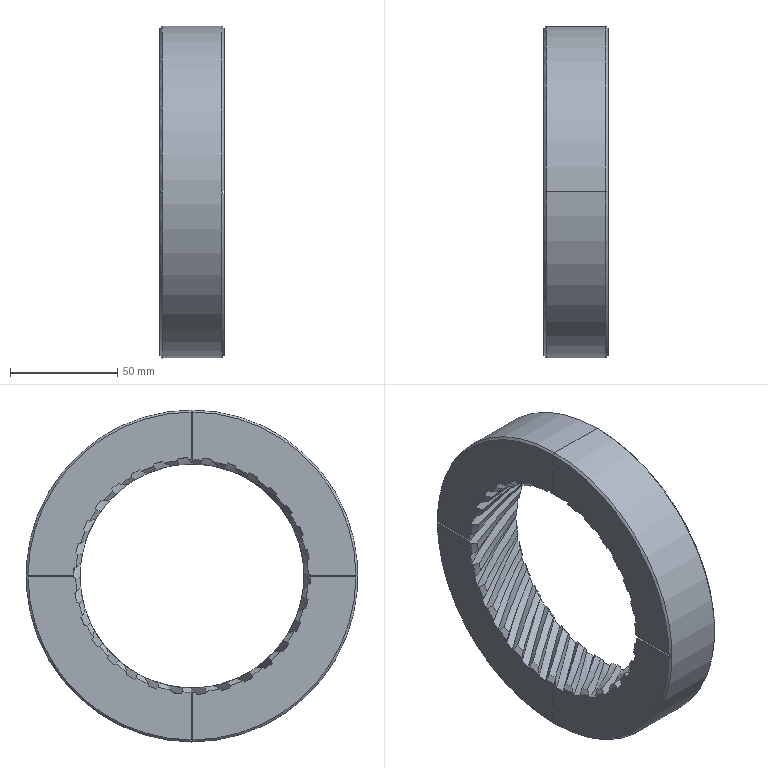Part | SolidWorks | features Chamfer 2, CirPattern 2, Extrusion 1, Helix 1, ICE 1, SweepCut 1 | 1 solid | 214 faces | box 30 x 155 x 155 mm | volume 292361 mm3 | spline 90 | cone 66 | cylinder 34 | plane 24 | commonest cylinder face diameters 104.5 x32 155 x2